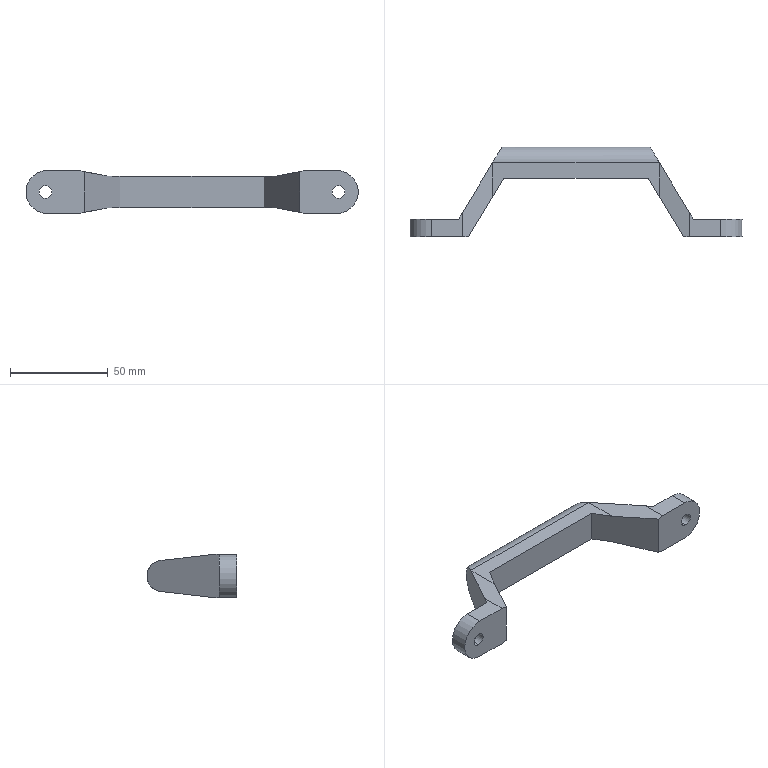Part | NX | features BREP 1 | 1 solid | 34 faces | box 170 x 46 x 22 mm | volume 38783 mm3 | plane 23 | cylinder 7 | cone 4 | commonest cylinder face diameters 6.5 x4 22 x2 16 x1
STEP:
#1=CARTESIAN_POINT('',(-75.,4.5,-3.25));
#2=VERTEX_POINT('',#1);
#3=CARTESIAN_POINT('',(-75.,4.5,3.25));
#4=VERTEX_POINT('',#3);
#5=CARTESIAN_POINT('',(-75.,4.5,0.));
#6=DIRECTION('',(0.,1.,0.));
#7=DIRECTION('',(0.,0.,1.));
#8=AXIS2_PLACEMENT_3D('',#5,#6,#7);
#9=CIRCLE('',#8,3.25);
#10=EDGE_CURVE('',#2,#4,#9,.T.);
#11=ORIENTED_EDGE('',*,*,#10,.F.);
#12=CARTESIAN_POINT('',(-75.,9.,-6.25));
#13=VERTEX_POINT('',#12);
#14=CARTESIAN_POINT('',(-75.,9.,-6.25));
#15=DIRECTION('',(0.,0.8321,-0.5547));
#16=VECTOR('',#15,1000.);
#17=LINE('',#14,#16);
#18=EDGE_CURVE('',#13,#2,#17,.F.);
#19=ORIENTED_EDGE('',*,*,#18,.F.);
#20=CARTESIAN_POINT('',(-75.,9.,6.25));
#21=VERTEX_POINT('',#20);
#22=CARTESIAN_POINT('',(-75.,9.,0.));
#23=DIRECTION('',(0.,-1.,0.));
#24=DIRECTION('',(0.,0.,1.));
#25=AXIS2_PLACEMENT_3D('',#22,#23,#24);
#26=CIRCLE('',#25,6.25);
#27=EDGE_CURVE('',#21,#13,#26,.T.);
#28=ORIENTED_EDGE('',*,*,#27,.F.);
#29=CARTESIAN_POINT('',(-75.,9.,6.25));
#30=DIRECTION('',(0.,0.8321,0.5547));
#31=VECTOR('',#30,1000.);
#32=LINE('',#29,#31);
#33=EDGE_CURVE('',#21,#4,#32,.F.);
#34=ORIENTED_EDGE('',*,*,#33,.T.);
#35=EDGE_LOOP('',(#11,#19,#28,#34));
#36=FACE_BOUND('',#35,.T.);
#37=CARTESIAN_POINT('',(-75.,9.,0.));
#38=DIRECTION('',(0.,1.,0.));
#39=DIRECTION('',(0.,0.,1.));
#40=AXIS2_PLACEMENT_3D('',#37,#38,#39);
#41=CONICAL_SURFACE('',#40,6.25,0.588);
#42=ADVANCED_FACE('',(#36),#41,.F.);
#43=CARTESIAN_POINT('',(75.,4.5,-3.25));
#44=VERTEX_POINT('',#43);
#45=CARTESIAN_POINT('',(75.,4.5,3.25));
#46=VERTEX_POINT('',#45);
#47=CARTESIAN_POINT('',(75.,4.5,0.));
#48=DIRECTION('',(0.,1.,0.));
#49=DIRECTION('',(0.,0.,1.));
#50=AXIS2_PLACEMENT_3D('',#47,#48,#49);
#51=CIRCLE('',#50,3.25);
#52=EDGE_CURVE('',#44,#46,#51,.T.);
#53=ORIENTED_EDGE('',*,*,#52,.F.);
#54=CARTESIAN_POINT('',(75.,9.,-6.25));
#55=VERTEX_POINT('',#54);
#56=CARTESIAN_POINT('',(75.,9.,-6.25));
#57=DIRECTION('',(0.,0.8321,-0.5547));
#58=VECTOR('',#57,1000.);
#59=LINE('',#56,#58);
#60=EDGE_CURVE('',#55,#44,#59,.F.);
#61=ORIENTED_EDGE('',*,*,#60,.F.);
#62=CARTESIAN_POINT('',(75.,9.,6.25));
#63=VERTEX_POINT('',#62);
#64=CARTESIAN_POINT('',(75.,9.,0.));
#65=DIRECTION('',(0.,-1.,0.));
#66=DIRECTION('',(0.,0.,1.));
#67=AXIS2_PLACEMENT_3D('',#64,#65,#66);
#68=CIRCLE('',#67,6.25);
#69=EDGE_CURVE('',#63,#55,#68,.T.);
#70=ORIENTED_EDGE('',*,*,#69,.F.);
#71=CARTESIAN_POINT('',(75.,9.,6.25));
#72=DIRECTION('',(0.,0.8321,0.5547));
#73=VECTOR('',#72,1000.);
#74=LINE('',#71,#73);
#75=EDGE_CURVE('',#63,#46,#74,.F.);
#76=ORIENTED_EDGE('',*,*,#75,.T.);
#77=EDGE_LOOP('',(#53,#61,#70,#76));
#78=FACE_BOUND('',#77,.T.);
#79=CARTESIAN_POINT('',(75.,9.,0.));
#80=DIRECTION('',(0.,1.,0.));
#81=DIRECTION('',(0.,0.,1.));
#82=AXIS2_PLACEMENT_3D('',#79,#80,#81);
#83=CONICAL_SURFACE('',#82,6.25,0.588);
#84=ADVANCED_FACE('',(#78),#83,.F.);
#85=ORIENTED_EDGE('',*,*,#10,.T.);
#86=CARTESIAN_POINT('',(-75.,0.,3.25));
#87=VERTEX_POINT('',#86);
#88=CARTESIAN_POINT('',(-75.,2.25,3.25));
#89=DIRECTION('',(0.,-1.,0.));
#90=VECTOR('',#89,1000.);
#91=LINE('',#88,#90);
#92=EDGE_CURVE('',#4,#87,#91,.T.);
#93=ORIENTED_EDGE('',*,*,#92,.T.);
#94=CARTESIAN_POINT('',(-75.,0.,-3.25));
#95=VERTEX_POINT('',#94);
#96=CARTESIAN_POINT('',(-75.,0.,0.));
#97=DIRECTION('',(0.,1.,0.));
#98=DIRECTION('',(0.,0.,-1.));
#99=AXIS2_PLACEMENT_3D('',#96,#97,#98);
#100=CIRCLE('',#99,3.25);
#101=EDGE_CURVE('',#95,#87,#100,.T.);
#102=ORIENTED_EDGE('',*,*,#101,.F.);
#103=CARTESIAN_POINT('',(-75.,2.25,-3.25));
#104=DIRECTION('',(0.,-1.,0.));
#105=VECTOR('',#104,1000.);
#106=LINE('',#103,#105);
#107=EDGE_CURVE('',#2,#95,#106,.T.);
#108=ORIENTED_EDGE('',*,*,#107,.F.);
#109=EDGE_LOOP('',(#85,#93,#102,#108));
#110=FACE_BOUND('',#109,.T.);
#111=CARTESIAN_POINT('',(-75.,2.25,0.));
#112=DIRECTION('',(0.,-1.,0.));
#113=DIRECTION('',(0.,0.,-1.));
#114=AXIS2_PLACEMENT_3D('',#111,#112,#113);
#115=CYLINDRICAL_SURFACE('',#114,3.25);
#116=ADVANCED_FACE('',(#110),#115,.F.);
#117=ORIENTED_EDGE('',*,*,#52,.T.);
#118=CARTESIAN_POINT('',(75.,0.,3.25));
#119=VERTEX_POINT('',#118);
#120=CARTESIAN_POINT('',(75.,2.25,3.25));
#121=DIRECTION('',(0.,-1.,0.));
#122=VECTOR('',#121,1000.);
#123=LINE('',#120,#122);
#124=EDGE_CURVE('',#46,#119,#123,.T.);
#125=ORIENTED_EDGE('',*,*,#124,.T.);
#126=CARTESIAN_POINT('',(75.,0.,-3.25));
#127=VERTEX_POINT('',#126);
#128=CARTESIAN_POINT('',(75.,0.,0.));
#129=DIRECTION('',(0.,1.,0.));
#130=DIRECTION('',(0.,0.,-1.));
#131=AXIS2_PLACEMENT_3D('',#128,#129,#130);
#132=CIRCLE('',#131,3.25);
#133=EDGE_CURVE('',#127,#119,#132,.T.);
#134=ORIENTED_EDGE('',*,*,#133,.F.);
#135=CARTESIAN_POINT('',(75.,2.25,-3.25));
#136=DIRECTION('',(0.,-1.,0.));
#137=VECTOR('',#136,1000.);
#138=LINE('',#135,#137);
#139=EDGE_CURVE('',#44,#127,#138,.T.);
#140=ORIENTED_EDGE('',*,*,#139,.F.);
#141=EDGE_LOOP('',(#117,#125,#134,#140));
#142=FACE_BOUND('',#141,.T.);
#143=CARTESIAN_POINT('',(75.,2.25,0.));
#144=DIRECTION('',(0.,-1.,0.));
#145=DIRECTION('',(0.,0.,-1.));
#146=AXIS2_PLACEMENT_3D('',#143,#144,#145);
#147=CYLINDRICAL_SURFACE('',#146,3.25);
#148=ADVANCED_FACE('',(#142),#147,.F.);
#149=CARTESIAN_POINT('',(-42.667,38.,-8.));
#150=VERTEX_POINT('',#149);
#151=CARTESIAN_POINT('',(-42.667,38.,8.));
#152=VERTEX_POINT('',#151);
#153=CARTESIAN_POINT('',(-42.667,38.,-8.));
#154=CARTESIAN_POINT('',(-33.053,54.,-8.));
#155=CARTESIAN_POINT('',(-33.053,54.,8.));
#156=CARTESIAN_POINT('',(-42.667,38.,8.));
#157=(BOUNDED_CURVE()B_SPLINE_CURVE(3,(#153,#154,#155,#156),.UNSPECIFIED.,.F.,.F.)B_SPLINE_CURVE_WITH_KNOTS((4,4),(4.712,7.854),.UNSPECIFIED.)CURVE()GEOMETRIC_REPRESENTATION_ITEM()RATIONAL_B_SPLINE_CURVE((1.,0.3333,0.3333,1.))REPRESENTATION_ITEM(''));
#158=EDGE_CURVE('',#150,#152,#157,.T.);
#159=ORIENTED_EDGE('',*,*,#158,.T.);
#160=CARTESIAN_POINT('',(-42.566,38.,8.));
#161=VERTEX_POINT('',#160);
#162=CARTESIAN_POINT('',(85.,38.,8.));
#163=DIRECTION('',(1.,0.,0.));
#164=VECTOR('',#163,1000.);
#165=LINE('',#162,#164);
#166=EDGE_CURVE('',#152,#161,#165,.T.);
#167=ORIENTED_EDGE('',*,*,#166,.T.);
#168=CARTESIAN_POINT('',(42.566,38.,8.));
#169=VERTEX_POINT('',#168);
#170=CARTESIAN_POINT('',(85.,38.,8.));
#171=DIRECTION('',(1.,0.,0.));
#172=VECTOR('',#171,1000.);
#173=LINE('',#170,#172);
#174=EDGE_CURVE('',#161,#169,#173,.T.);
#175=ORIENTED_EDGE('',*,*,#174,.T.);
#176=CARTESIAN_POINT('',(42.667,38.,8.));
#177=VERTEX_POINT('',#176);
#178=CARTESIAN_POINT('',(85.,38.,8.));
#179=DIRECTION('',(1.,0.,0.));
#180=VECTOR('',#179,1000.);
#181=LINE('',#178,#180);
#182=EDGE_CURVE('',#169,#177,#181,.T.);
#183=ORIENTED_EDGE('',*,*,#182,.T.);
#184=CARTESIAN_POINT('',(42.667,38.,-8.));
#185=VERTEX_POINT('',#184);
#186=CARTESIAN_POINT('',(42.667,38.,8.));
#187=CARTESIAN_POINT('',(33.053,54.,8.));
#188=CARTESIAN_POINT('',(33.053,54.,-8.));
#189=CARTESIAN_POINT('',(42.667,38.,-8.));
#190=(BOUNDED_CURVE()B_SPLINE_CURVE(3,(#186,#187,#188,#189),.UNSPECIFIED.,.F.,.F.)B_SPLINE_CURVE_WITH_KNOTS((4,4),(1.571,4.712),.UNSPECIFIED.)CURVE()GEOMETRIC_REPRESENTATION_ITEM()RATIONAL_B_SPLINE_CURVE((1.,0.3333,0.3333,1.))REPRESENTATION_ITEM(''));
#191=EDGE_CURVE('',#177,#185,#190,.T.);
#192=ORIENTED_EDGE('',*,*,#191,.T.);
#193=CARTESIAN_POINT('',(42.566,38.,-8.));
#194=VERTEX_POINT('',#193);
#195=CARTESIAN_POINT('',(85.,38.,-8.));
#196=DIRECTION('',(-1.,0.,0.));
#197=VECTOR('',#196,1000.);
#198=LINE('',#195,#197);
#199=EDGE_CURVE('',#185,#194,#198,.T.);
#200=ORIENTED_EDGE('',*,*,#199,.T.);
#201=CARTESIAN_POINT('',(-42.566,38.,-8.));
#202=VERTEX_POINT('',#201);
#203=CARTESIAN_POINT('',(85.,38.,-8.));
#204=DIRECTION('',(-1.,0.,0.));
#205=VECTOR('',#204,1000.);
#206=LINE('',#203,#205);
#207=EDGE_CURVE('',#194,#202,#206,.T.);
#208=ORIENTED_EDGE('',*,*,#207,.T.);
#209=CARTESIAN_POINT('',(85.,38.,-8.));
#210=DIRECTION('',(-1.,0.,0.));
#211=VECTOR('',#210,1000.);
#212=LINE('',#209,#211);
#213=EDGE_CURVE('',#202,#150,#212,.T.);
#214=ORIENTED_EDGE('',*,*,#213,.T.);
#215=EDGE_LOOP('',(#159,#167,#175,#183,#192,#200,#208,#214));
#216=FACE_BOUND('',#215,.T.);
#217=CARTESIAN_POINT('',(85.,38.,0.));
#218=DIRECTION('',(1.,0.,0.));
#219=DIRECTION('',(0.,0.,-1.));
#220=AXIS2_PLACEMENT_3D('',#217,#218,#219);
#221=CYLINDRICAL_SURFACE('',#220,8.);
#222=ADVANCED_FACE('',(#216),#221,.T.);
#223=CARTESIAN_POINT('',(-42.667,38.,8.02));
#224=VERTEX_POINT('',#223);
#225=CARTESIAN_POINT('',(-42.667,38.,9.9));
#226=DIRECTION('',(0.,0.,-1.));
#227=VECTOR('',#226,1000.);
#228=LINE('',#225,#227);
#229=EDGE_CURVE('',#224,#152,#228,.T.);
#230=ORIENTED_EDGE('',*,*,#229,.F.);
#231=CARTESIAN_POINT('',(-42.566,38.,8.));
#232=DIRECTION('',(0.9816,0.,-0.1908));
#233=VECTOR('',#232,1000.);
#234=LINE('',#231,#233);
#235=EDGE_CURVE('',#224,#161,#234,.T.);
#236=ORIENTED_EDGE('',*,*,#235,.T.);
#237=ORIENTED_EDGE('',*,*,#166,.F.);
#238=EDGE_LOOP('',(#230,#236,#237));
#239=FACE_BOUND('',#238,.T.);
#240=CARTESIAN_POINT('',(85.,38.,9.9));
#241=DIRECTION('',(0.,-1.,0.));
#242=DIRECTION('',(-1.,0.,0.));
#243=AXIS2_PLACEMENT_3D('',#240,#241,#242);
#244=PLANE('',#243);
#245=ADVANCED_FACE('',(#239),#244,.F.);
#246=CARTESIAN_POINT('',(-58.,12.482,-11.));
#247=VERTEX_POINT('',#246);
#248=CARTESIAN_POINT('',(-60.092,9.,-11.));
#249=VERTEX_POINT('',#248);
#250=CARTESIAN_POINT('',(-37.86,46.,-11.));
#251=DIRECTION('',(-0.515,-0.8572,0.));
#252=VECTOR('',#251,1000.);
#253=LINE('',#250,#252);
#254=EDGE_CURVE('',#247,#249,#253,.T.);
#255=ORIENTED_EDGE('',*,*,#254,.T.);
#256=CARTESIAN_POINT('',(-60.092,9.,11.));
#257=VERTEX_POINT('',#256);
#258=CARTESIAN_POINT('',(-60.092,9.,11.));
#259=DIRECTION('',(0.,0.,1.));
#260=VECTOR('',#259,1000.);
#261=LINE('',#258,#260);
#262=EDGE_CURVE('',#249,#257,#261,.T.);
#263=ORIENTED_EDGE('',*,*,#262,.T.);
#264=CARTESIAN_POINT('',(-58.,12.482,11.));
#265=VERTEX_POINT('',#264);
#266=CARTESIAN_POINT('',(-37.86,46.,11.));
#267=DIRECTION('',(0.515,0.8572,0.));
#268=VECTOR('',#267,1000.);
#269=LINE('',#266,#268);
#270=EDGE_CURVE('',#257,#265,#269,.T.);
#271=ORIENTED_EDGE('',*,*,#270,.T.);
#272=CARTESIAN_POINT('',(-58.,12.482,11.));
#273=DIRECTION('',(0.5125,0.8529,-0.09962));
#274=VECTOR('',#273,1000.);
#275=LINE('',#272,#274);
#276=EDGE_CURVE('',#265,#224,#275,.T.);
#277=ORIENTED_EDGE('',*,*,#276,.T.);
#278=ORIENTED_EDGE('',*,*,#229,.T.);
#279=ORIENTED_EDGE('',*,*,#158,.F.);
#280=CARTESIAN_POINT('',(-42.667,38.,-8.02));
#281=VERTEX_POINT('',#280);
#282=CARTESIAN_POINT('',(-42.667,38.,11.));
#283=DIRECTION('',(0.,0.,-1.));
#284=VECTOR('',#283,1000.);
#285=LINE('',#282,#284);
#286=EDGE_CURVE('',#150,#281,#285,.T.);
#287=ORIENTED_EDGE('',*,*,#286,.T.);
#288=CARTESIAN_POINT('',(-42.667,38.,-8.02));
#289=DIRECTION('',(-0.5125,-0.8529,-0.09962));
#290=VECTOR('',#289,1000.);
#291=LINE('',#288,#290);
#292=EDGE_CURVE('',#281,#247,#291,.T.);
#293=ORIENTED_EDGE('',*,*,#292,.T.);
#294=EDGE_LOOP('',(#255,#263,#271,#277,#278,#279,#287,#293));
#295=FACE_BOUND('',#294,.T.);
#296=CARTESIAN_POINT('',(-37.86,46.,11.));
#297=DIRECTION('',(-0.8572,0.515,0.));
#298=DIRECTION('',(0.,0.,1.));
#299=AXIS2_PLACEMENT_3D('',#296,#297,#298);
#300=PLANE('',#299);
#301=ADVANCED_FACE('',(#295),#300,.T.);
#302=CARTESIAN_POINT('',(-42.667,38.,-8.02));
#303=DIRECTION('',(0.9816,0.,0.1908));
#304=VECTOR('',#303,1000.);
#305=LINE('',#302,#304);
#306=EDGE_CURVE('',#281,#202,#305,.T.);
#307=ORIENTED_EDGE('',*,*,#306,.F.);
#308=ORIENTED_EDGE('',*,*,#286,.F.);
#309=ORIENTED_EDGE('',*,*,#213,.F.);
#310=EDGE_LOOP('',(#307,#308,#309));
#311=FACE_BOUND('',#310,.T.);
#312=CARTESIAN_POINT('',(85.,38.,-8.));
#313=DIRECTION('',(0.,-1.,0.));
#314=DIRECTION('',(0.,0.,-1.));
#315=AXIS2_PLACEMENT_3D('',#312,#313,#314);
#316=PLANE('',#315);
#317=ADVANCED_FACE('',(#311),#316,.F.);
#318=CARTESIAN_POINT('',(36.974,30.,-8.));
#319=VERTEX_POINT('',#318);
#320=CARTESIAN_POINT('',(42.566,20.693,-8.));
#321=VERTEX_POINT('',#320);
#322=CARTESIAN_POINT('',(36.974,30.,-8.));
#323=DIRECTION('',(0.515,-0.8572,0.));
#324=VECTOR('',#323,1000.);
#325=LINE('',#322,#324);
#326=EDGE_CURVE('',#319,#321,#325,.T.);
#327=ORIENTED_EDGE('',*,*,#326,.F.);
#328=CARTESIAN_POINT('',(-36.974,30.,-8.));
#329=VERTEX_POINT('',#328);
#330=CARTESIAN_POINT('',(-42.566,30.,-8.));
#331=DIRECTION('',(1.,0.,0.));
#332=VECTOR('',#331,1000.);
#333=LINE('',#330,#332);
#334=EDGE_CURVE('',#329,#319,#333,.T.);
#335=ORIENTED_EDGE('',*,*,#334,.F.);
#336=CARTESIAN_POINT('',(-42.566,20.693,-8.));
#337=VERTEX_POINT('',#336);
#338=CARTESIAN_POINT('',(-42.566,20.693,-8.));
#339=DIRECTION('',(0.515,0.8572,0.));
#340=VECTOR('',#339,1000.);
#341=LINE('',#338,#340);
#342=EDGE_CURVE('',#337,#329,#341,.T.);
#343=ORIENTED_EDGE('',*,*,#342,.F.);
#344=CARTESIAN_POINT('',(-42.566,46.,-8.));
#345=DIRECTION('',(0.,-1.,0.));
#346=VECTOR('',#345,1000.);
#347=LINE('',#344,#346);
#348=EDGE_CURVE('',#202,#337,#347,.T.);
#349=ORIENTED_EDGE('',*,*,#348,.F.);
#350=ORIENTED_EDGE('',*,*,#207,.F.);
#351=CARTESIAN_POINT('',(42.566,46.,-8.));
#352=DIRECTION('',(0.,1.,0.));
#353=VECTOR('',#352,1000.);
#354=LINE('',#351,#353);
#355=EDGE_CURVE('',#321,#194,#354,.T.);
#356=ORIENTED_EDGE('',*,*,#355,.F.);
#357=EDGE_LOOP('',(#327,#335,#343,#349,#350,#356));
#358=FACE_BOUND('',#357,.T.);
#359=CARTESIAN_POINT('',(-42.566,46.,-8.));
#360=DIRECTION('',(0.,0.,1.));
#361=DIRECTION('',(1.,0.,0.));
#362=AXIS2_PLACEMENT_3D('',#359,#360,#361);
#363=PLANE('',#362);
#364=ADVANCED_FACE('',(#358),#363,.F.);
#365=ORIENTED_EDGE('',*,*,#199,.F.);
#366=CARTESIAN_POINT('',(42.667,38.,-8.02));
#367=VERTEX_POINT('',#366);
#368=CARTESIAN_POINT('',(42.667,38.,-8.));
#369=DIRECTION('',(0.,0.,1.));
#370=VECTOR('',#369,1000.);
#371=LINE('',#368,#370);
#372=EDGE_CURVE('',#367,#185,#371,.T.);
#373=ORIENTED_EDGE('',*,*,#372,.F.);
#374=CARTESIAN_POINT('',(42.566,38.,-8.));
#375=DIRECTION('',(0.9816,0.,-0.1908));
#376=VECTOR('',#375,1000.);
#377=LINE('',#374,#376);
#378=EDGE_CURVE('',#194,#367,#377,.T.);
#379=ORIENTED_EDGE('',*,*,#378,.F.);
#380=EDGE_LOOP('',(#365,#373,#379));
#381=FACE_BOUND('',#380,.T.);
#382=CARTESIAN_POINT('',(85.,38.,-8.));
#383=DIRECTION('',(0.,-1.,0.));
#384=DIRECTION('',(0.,0.,-1.));
#385=AXIS2_PLACEMENT_3D('',#382,#383,#384);
#386=PLANE('',#385);
#387=ADVANCED_FACE('',(#381),#386,.F.);
#388=CARTESIAN_POINT('',(60.092,9.,-11.));
#389=VERTEX_POINT('',#388);
#390=CARTESIAN_POINT('',(58.,12.482,-11.));
#391=VERTEX_POINT('',#390);
#392=CARTESIAN_POINT('',(60.092,9.,-11.));
#393=DIRECTION('',(-0.515,0.8572,0.));
#394=VECTOR('',#393,1000.);
#395=LINE('',#392,#394);
#396=EDGE_CURVE('',#389,#391,#395,.T.);
#397=ORIENTED_EDGE('',*,*,#396,.T.);
#398=CARTESIAN_POINT('',(58.,12.482,-11.));
#399=DIRECTION('',(-0.5125,0.8529,0.09962));
#400=VECTOR('',#399,1000.);
#401=LINE('',#398,#400);
#402=EDGE_CURVE('',#391,#367,#401,.T.);
#403=ORIENTED_EDGE('',*,*,#402,.T.);
#404=ORIENTED_EDGE('',*,*,#372,.T.);
#405=ORIENTED_EDGE('',*,*,#191,.F.);
#406=CARTESIAN_POINT('',(42.667,38.,8.02));
#407=VERTEX_POINT('',#406);
#408=CARTESIAN_POINT('',(42.667,38.,11.));
#409=DIRECTION('',(0.,0.,1.));
#410=VECTOR('',#409,1000.);
#411=LINE('',#408,#410);
#412=EDGE_CURVE('',#177,#407,#411,.T.);
#413=ORIENTED_EDGE('',*,*,#412,.T.);
#414=CARTESIAN_POINT('',(58.,12.482,11.));
#415=VERTEX_POINT('',#414);
#416=CARTESIAN_POINT('',(42.667,38.,8.02));
#417=DIRECTION('',(0.5125,-0.8529,0.09962));
#418=VECTOR('',#417,1000.);
#419=LINE('',#416,#418);
#420=EDGE_CURVE('',#407,#415,#419,.T.);
#421=ORIENTED_EDGE('',*,*,#420,.T.);
#422=CARTESIAN_POINT('',(60.092,9.,11.));
#423=VERTEX_POINT('',#422);
#424=CARTESIAN_POINT('',(60.092,9.,11.));
#425=DIRECTION('',(0.515,-0.8572,0.));
#426=VECTOR('',#425,1000.);
#427=LINE('',#424,#426);
#428=EDGE_CURVE('',#415,#423,#427,.T.);
#429=ORIENTED_EDGE('',*,*,#428,.T.);
#430=CARTESIAN_POINT('',(60.092,9.,11.));
#431=DIRECTION('',(0.,0.,-1.));
#432=VECTOR('',#431,1000.);
#433=LINE('',#430,#432);
#434=EDGE_CURVE('',#423,#389,#433,.T.);
#435=ORIENTED_EDGE('',*,*,#434,.T.);
#436=EDGE_LOOP('',(#397,#403,#404,#405,#413,#421,#429,#435));
#437=FACE_BOUND('',#436,.T.);
#438=CARTESIAN_POINT('',(60.092,9.,11.));
#439=DIRECTION('',(0.8572,0.515,0.));
#440=DIRECTION('',(0.,0.,-1.));
#441=AXIS2_PLACEMENT_3D('',#438,#439,#440);
#442=PLANE('',#441);
#443=ADVANCED_FACE('',(#437),#442,.T.);
#444=ORIENTED_EDGE('',*,*,#182,.F.);
#445=CARTESIAN_POINT('',(42.667,38.,8.02));
#446=DIRECTION('',(-0.9816,0.,-0.1908));
#447=VECTOR('',#446,1000.);
#448=LINE('',#445,#447);
#449=EDGE_CURVE('',#407,#169,#448,.T.);
#450=ORIENTED_EDGE('',*,*,#449,.F.);
#451=ORIENTED_EDGE('',*,*,#412,.F.);
#452=EDGE_LOOP('',(#444,#450,#451));
#453=FACE_BOUND('',#452,.T.);
#454=CARTESIAN_POINT('',(85.,38.,9.9));
#455=DIRECTION('',(0.,-1.,0.));
#456=DIRECTION('',(-1.,0.,0.));
#457=AXIS2_PLACEMENT_3D('',#454,#455,#456);
#458=PLANE('',#457);
#459=ADVANCED_FACE('',(#453),#458,.F.);
#460=CARTESIAN_POINT('',(-36.974,30.,8.));
#461=VERTEX_POINT('',#460);
#462=CARTESIAN_POINT('',(-42.566,20.693,8.));
#463=VERTEX_POINT('',#462);
#464=CARTESIAN_POINT('',(-36.974,30.,8.));
#465=DIRECTION('',(-0.515,-0.8572,0.));
#466=VECTOR('',#465,1000.);
#467=LINE('',#464,#466);
#468=EDGE_CURVE('',#461,#463,#467,.T.);
#469=ORIENTED_EDGE('',*,*,#468,.F.);
#470=CARTESIAN_POINT('',(36.974,30.,8.));
#471=VERTEX_POINT('',#470);
#472=CARTESIAN_POINT('',(42.566,30.,8.));
#473=DIRECTION('',(-1.,0.,0.));
#474=VECTOR('',#473,1000.);
#475=LINE('',#472,#474);
#476=EDGE_CURVE('',#471,#461,#475,.T.);
#477=ORIENTED_EDGE('',*,*,#476,.F.);
#478=CARTESIAN_POINT('',(42.566,20.693,8.));
#479=VERTEX_POINT('',#478);
#480=CARTESIAN_POINT('',(42.566,20.693,8.));
#481=DIRECTION('',(-0.515,0.8572,0.));
#482=VECTOR('',#481,1000.);
#483=LINE('',#480,#482);
#484=EDGE_CURVE('',#479,#471,#483,.T.);
#485=ORIENTED_EDGE('',*,*,#484,.F.);
#486=CARTESIAN_POINT('',(42.566,46.,8.));
#487=DIRECTION('',(0.,-1.,0.));
#488=VECTOR('',#487,1000.);
#489=LINE('',#486,#488);
#490=EDGE_CURVE('',#169,#479,#489,.T.);
#491=ORIENTED_EDGE('',*,*,#490,.F.);
#492=ORIENTED_EDGE('',*,*,#174,.F.);
#493=CARTESIAN_POINT('',(-42.566,46.,8.));
#494=DIRECTION('',(0.,1.,0.));
#495=VECTOR('',#494,1000.);
#496=LINE('',#493,#495);
#497=EDGE_CURVE('',#463,#161,#496,.T.);
#498=ORIENTED_EDGE('',*,*,#497,.F.);
#499=EDGE_LOOP('',(#469,#477,#485,#491,#492,#498));
#500=FACE_BOUND('',#499,.T.);
#501=CARTESIAN_POINT('',(42.566,46.,8.));
#502=DIRECTION('',(0.,0.,-1.));
#503=DIRECTION('',(0.,-1.,0.));
#504=AXIS2_PLACEMENT_3D('',#501,#502,#503);
#505=PLANE('',#504);
#506=ADVANCED_FACE('',(#500),#505,.F.);
#507=CARTESIAN_POINT('',(-74.,9.,-11.));
#508=VERTEX_POINT('',#507);
#509=CARTESIAN_POINT('',(-74.,9.,11.));
#510=VERTEX_POINT('',#509);
#511=CARTESIAN_POINT('',(-74.,9.,0.));
#512=DIRECTION('',(0.,1.,0.));
#513=DIRECTION('',(0.,0.,-1.));
#514=AXIS2_PLACEMENT_3D('',#511,#512,#513);
#515=CIRCLE('',#514,11.);
#516=EDGE_CURVE('',#508,#510,#515,.T.);
#517=ORIENTED_EDGE('',*,*,#516,.T.);
#518=CARTESIAN_POINT('',(-60.092,9.,11.));
#519=DIRECTION('',(1.,0.,0.));
#520=VECTOR('',#519,1000.);
#521=LINE('',#518,#520);
#522=EDGE_CURVE('',#510,#257,#521,.T.);
#523=ORIENTED_EDGE('',*,*,#522,.T.);
#524=ORIENTED_EDGE('',*,*,#262,.F.);
#525=CARTESIAN_POINT('',(-60.092,9.,-11.));
#526=DIRECTION('',(-1.,0.,0.));
#527=VECTOR('',#526,1000.);
#528=LINE('',#525,#527);
#529=EDGE_CURVE('',#249,#508,#528,.T.);
#530=ORIENTED_EDGE('',*,*,#529,.T.);
#531=EDGE_LOOP('',(#517,#523,#524,#530));
#532=FACE_BOUND('',#531,.T.);
#533=ORIENTED_EDGE('',*,*,#27,.T.);
#534=CARTESIAN_POINT('',(-75.,9.,0.));
#535=DIRECTION('',(0.,-1.,0.));
#536=DIRECTION('',(0.,0.,1.));
#537=AXIS2_PLACEMENT_3D('',#534,#535,#536);
#538=CIRCLE('',#537,6.25);
#539=EDGE_CURVE('',#13,#21,#538,.T.);
#540=ORIENTED_EDGE('',*,*,#539,.T.);
#541=EDGE_LOOP('',(#533,#540));
#542=FACE_BOUND('',#541,.T.);
#543=CARTESIAN_POINT('',(-60.092,9.,11.));
#544=DIRECTION('',(0.,1.,0.));
#545=DIRECTION('',(1.,0.,0.));
#546=AXIS2_PLACEMENT_3D('',#543,#544,#545);
#547=PLANE('',#546);
#548=ADVANCED_FACE('',(#532,#542),#547,.T.);
#549=ORIENTED_EDGE('',*,*,#254,.F.);
#550=CARTESIAN_POINT('',(-58.,0.,-11.));
#551=VERTEX_POINT('',#550);
#552=CARTESIAN_POINT('',(-58.,0.,-11.));
#553=DIRECTION('',(0.,1.,0.));
#554=VECTOR('',#553,1000.);
#555=LINE('',#552,#554);
#556=EDGE_CURVE('',#551,#247,#555,.T.);
#557=ORIENTED_EDGE('',*,*,#556,.F.);
#558=CARTESIAN_POINT('',(-74.,0.,-11.));
#559=VERTEX_POINT('',#558);
#560=CARTESIAN_POINT('',(0.,0.,-11.));
#561=DIRECTION('',(1.,0.,0.));
#562=VECTOR('',#561,1000.);
#563=LINE('',#560,#562);
#564=EDGE_CURVE('',#559,#551,#563,.T.);
#565=ORIENTED_EDGE('',*,*,#564,.F.);
#566=CARTESIAN_POINT('',(-74.,0.,-11.));
#567=DIRECTION('',(0.,-1.,0.));
#568=VECTOR('',#567,1000.);
#569=LINE('',#566,#568);
#570=EDGE_CURVE('',#508,#559,#569,.T.);
#571=ORIENTED_EDGE('',*,*,#570,.F.);
#572=ORIENTED_EDGE('',*,*,#529,.F.);
#573=EDGE_LOOP('',(#549,#557,#565,#571,#572));
#574=FACE_BOUND('',#573,.T.);
#575=CARTESIAN_POINT('',(0.,0.,-11.));
#576=DIRECTION('',(0.,0.,1.));
#577=DIRECTION('',(1.,0.,0.));
#578=AXIS2_PLACEMENT_3D('',#575,#576,#577);
#579=PLANE('',#578);
#580=ADVANCED_FACE('',(#574),#579,.F.);
#581=CARTESIAN_POINT('',(-55.,0.,-10.417));
#582=VERTEX_POINT('',#581);
#583=CARTESIAN_POINT('',(-55.,0.,-10.417));
#584=DIRECTION('',(0.5125,0.8529,0.09962));
#585=VECTOR('',#584,1000.);
#586=LINE('',#583,#585);
#587=EDGE_CURVE('',#582,#337,#586,.T.);
#588=ORIENTED_EDGE('',*,*,#587,.F.);
#589=CARTESIAN_POINT('',(-58.,0.,-11.));
#590=DIRECTION('',(0.9816,0.,0.1908));
#591=VECTOR('',#590,1000.);
#592=LINE('',#589,#591);
#593=EDGE_CURVE('',#551,#582,#592,.T.);
#594=ORIENTED_EDGE('',*,*,#593,.F.);
#595=ORIENTED_EDGE('',*,*,#556,.T.);
#596=ORIENTED_EDGE('',*,*,#292,.F.);
#597=ORIENTED_EDGE('',*,*,#306,.T.);
#598=ORIENTED_EDGE('',*,*,#348,.T.);
#599=EDGE_LOOP('',(#588,#594,#595,#596,#597,#598));
#600=FACE_BOUND('',#599,.T.);
#601=CARTESIAN_POINT('',(-58.,46.,-11.));
#602=DIRECTION('',(-0.1908,0.,0.9816));
#603=DIRECTION('',(0.,1.,0.));
#604=AXIS2_PLACEMENT_3D('',#601,#602,#603);
#605=PLANE('',#604);
#606=ADVANCED_FACE('',(#600),#605,.F.);
#607=CARTESIAN_POINT('',(-58.,0.,11.));
#608=VERTEX_POINT('',#607);
#609=CARTESIAN_POINT('',(-58.,46.,11.));
#610=DIRECTION('',(0.,1.,0.));
#611=VECTOR('',#610,1000.);
#612=LINE('',#609,#611);
#613=EDGE_CURVE('',#608,#265,#612,.T.);
#614=ORIENTED_EDGE('',*,*,#613,.F.);
#615=CARTESIAN_POINT('',(-55.,0.,10.417));
#616=VERTEX_POINT('',#615);
#617=CARTESIAN_POINT('',(-42.566,0.,8.));
#618=DIRECTION('',(-0.9816,0.,0.1908));
#619=VECTOR('',#618,1000.);
#620=LINE('',#617,#619);
#621=EDGE_CURVE('',#616,#608,#620,.T.);
#622=ORIENTED_EDGE('',*,*,#621,.F.);
#623=CARTESIAN_POINT('',(-42.566,20.693,8.));
#624=DIRECTION('',(-0.5125,-0.8529,0.09962));
#625=VECTOR('',#624,1000.);
#626=LINE('',#623,#625);
#627=EDGE_CURVE('',#463,#616,#626,.T.);
#628=ORIENTED_EDGE('',*,*,#627,.F.);
#629=ORIENTED_EDGE('',*,*,#497,.T.);
#630=ORIENTED_EDGE('',*,*,#235,.F.);
#631=ORIENTED_EDGE('',*,*,#276,.F.);
#632=EDGE_LOOP('',(#614,#622,#628,#629,#630,#631));
#633=FACE_BOUND('',#632,.T.);
#634=CARTESIAN_POINT('',(-42.566,46.,8.));
#635=DIRECTION('',(-0.1908,0.,-0.9816));
#636=DIRECTION('',(-0.9816,0.,0.1908));
#637=AXIS2_PLACEMENT_3D('',#634,#635,#636);
#638=PLANE('',#637);
#639=ADVANCED_FACE('',(#633),#638,.F.);
#640=CARTESIAN_POINT('',(-74.,0.,11.));
#641=VERTEX_POINT('',#640);
#642=CARTESIAN_POINT('',(0.,0.,11.));
#643=DIRECTION('',(1.,0.,0.));
#644=VECTOR('',#643,1000.);
#645=LINE('',#642,#644);
#646=EDGE_CURVE('',#641,#608,#645,.T.);
#647=ORIENTED_EDGE('',*,*,#646,.T.);
#648=ORIENTED_EDGE('',*,*,#613,.T.);
#649=ORIENTED_EDGE('',*,*,#270,.F.);
#650=ORIENTED_EDGE('',*,*,#522,.F.);
#651=CARTESIAN_POINT('',(-74.,0.,11.));
#652=DIRECTION('',(0.,-1.,0.));
#653=VECTOR('',#652,1000.);
#654=LINE('',#651,#653);
#655=EDGE_CURVE('',#510,#641,#654,.T.);
#656=ORIENTED_EDGE('',*,*,#655,.T.);
#657=EDGE_LOOP('',(#647,#648,#649,#650,#656));
#658=FACE_BOUND('',#657,.T.);
#659=CARTESIAN_POINT('',(0.,0.,11.));
#660=DIRECTION('',(0.,0.,1.));
#661=DIRECTION('',(1.,0.,0.));
#662=AXIS2_PLACEMENT_3D('',#659,#660,#661);
#663=PLANE('',#662);
#664=ADVANCED_FACE('',(#658),#663,.T.);
#665=CARTESIAN_POINT('',(58.,0.,-11.));
#666=VERTEX_POINT('',#665);
#667=CARTESIAN_POINT('',(58.,46.,-11.));
#668=DIRECTION('',(0.,1.,0.));
#669=VECTOR('',#668,1000.);
#670=LINE('',#667,#669);
#671=EDGE_CURVE('',#666,#391,#670,.T.);
#672=ORIENTED_EDGE('',*,*,#671,.F.);
#673=CARTESIAN_POINT('',(55.,0.,-10.417));
#674=VERTEX_POINT('',#673);
#675=CARTESIAN_POINT('',(42.566,0.,-8.));
#676=DIRECTION('',(0.9816,0.,-0.1908));
#677=VECTOR('',#676,1000.);
#678=LINE('',#675,#677);
#679=EDGE_CURVE('',#674,#666,#678,.T.);
#680=ORIENTED_EDGE('',*,*,#679,.F.);
#681=CARTESIAN_POINT('',(42.566,20.693,-8.));
#682=DIRECTION('',(0.5125,-0.8529,-0.09962));
#683=VECTOR('',#682,1000.);
#684=LINE('',#681,#683);
#685=EDGE_CURVE('',#321,#674,#684,.T.);
#686=ORIENTED_EDGE('',*,*,#685,.F.);
#687=ORIENTED_EDGE('',*,*,#355,.T.);
#688=ORIENTED_EDGE('',*,*,#378,.T.);
#689=ORIENTED_EDGE('',*,*,#402,.F.);
#690=EDGE_LOOP('',(#672,#680,#686,#687,#688,#689));
#691=FACE_BOUND('',#690,.T.);
#692=CARTESIAN_POINT('',(42.566,46.,-8.));
#693=DIRECTION('',(0.1908,0.,0.9816));
#694=DIRECTION('',(0.,-1.,0.));
#695=AXIS2_PLACEMENT_3D('',#692,#693,#694);
#696=PLANE('',#695);
#697=ADVANCED_FACE('',(#691),#696,.F.);
#698=CARTESIAN_POINT('',(36.974,30.,11.));
#699=DIRECTION('',(0.,0.,-1.));
#700=VECTOR('',#699,1000.);
#701=LINE('',#698,#700);
#702=EDGE_CURVE('',#471,#319,#701,.T.);
#703=ORIENTED_EDGE('',*,*,#702,.T.);
#704=ORIENTED_EDGE('',*,*,#326,.T.);
#705=ORIENTED_EDGE('',*,*,#685,.T.);
#706=CARTESIAN_POINT('',(55.,0.,10.417));
#707=VERTEX_POINT('',#706);
#708=CARTESIAN_POINT('',(55.,0.,11.));
#709=DIRECTION('',(0.,0.,1.));
#710=VECTOR('',#709,1000.);
#711=LINE('',#708,#710);
#712=EDGE_CURVE('',#674,#707,#711,.T.);
#713=ORIENTED_EDGE('',*,*,#712,.T.);
#714=CARTESIAN_POINT('',(55.,0.,10.417));
#715=DIRECTION('',(-0.5125,0.8529,-0.09962));
#716=VECTOR('',#715,1000.);
#717=LINE('',#714,#716);
#718=EDGE_CURVE('',#707,#479,#717,.T.);
#719=ORIENTED_EDGE('',*,*,#718,.T.);
#720=ORIENTED_EDGE('',*,*,#484,.T.);
#721=EDGE_LOOP('',(#703,#704,#705,#713,#719,#720));
#722=FACE_BOUND('',#721,.T.);
#723=CARTESIAN_POINT('',(36.974,30.,11.));
#724=DIRECTION('',(-0.8572,-0.515,0.));
#725=DIRECTION('',(-0.515,0.8572,0.));
#726=AXIS2_PLACEMENT_3D('',#723,#724,#725);
#727=PLANE('',#726);
#728=ADVANCED_FACE('',(#722),#727,.T.);
#729=ORIENTED_EDGE('',*,*,#476,.T.);
#730=CARTESIAN_POINT('',(-36.974,30.,11.));
#731=DIRECTION('',(0.,0.,-1.));
#732=VECTOR('',#731,1000.);
#733=LINE('',#730,#732);
#734=EDGE_CURVE('',#461,#329,#733,.T.);
#735=ORIENTED_EDGE('',*,*,#734,.T.);
#736=ORIENTED_EDGE('',*,*,#334,.T.);
#737=ORIENTED_EDGE('',*,*,#702,.F.);
#738=EDGE_LOOP('',(#729,#735,#736,#737));
#739=FACE_BOUND('',#738,.T.);
#740=CARTESIAN_POINT('',(-36.974,30.,11.));
#741=DIRECTION('',(0.,-1.,0.));
#742=DIRECTION('',(0.,0.,-1.));
#743=AXIS2_PLACEMENT_3D('',#740,#741,#742);
#744=PLANE('',#743);
#745=ADVANCED_FACE('',(#739),#744,.T.);
#746=ORIENTED_EDGE('',*,*,#587,.T.);
#747=ORIENTED_EDGE('',*,*,#342,.T.);
#748=ORIENTED_EDGE('',*,*,#734,.F.);
#749=ORIENTED_EDGE('',*,*,#468,.T.);
#750=ORIENTED_EDGE('',*,*,#627,.T.);
#751=CARTESIAN_POINT('',(-55.,0.,11.));
#752=DIRECTION('',(0.,0.,-1.));
#753=VECTOR('',#752,1000.);
#754=LINE('',#751,#753);
#755=EDGE_CURVE('',#616,#582,#754,.T.);
#756=ORIENTED_EDGE('',*,*,#755,.T.);
#757=EDGE_LOOP('',(#746,#747,#748,#749,#750,#756));
#758=FACE_BOUND('',#757,.T.);
#759=CARTESIAN_POINT('',(-55.,0.,11.));
#760=DIRECTION('',(0.8572,-0.515,0.));
#761=DIRECTION('',(0.,0.,-1.));
#762=AXIS2_PLACEMENT_3D('',#759,#760,#761);
#763=PLANE('',#762);
#764=ADVANCED_FACE('',(#758),#763,.T.);
#765=ORIENTED_EDGE('',*,*,#671,.T.);
#766=ORIENTED_EDGE('',*,*,#396,.F.);
#767=CARTESIAN_POINT('',(74.,9.,-11.));
#768=VERTEX_POINT('',#767);
#769=CARTESIAN_POINT('',(0.,9.,-11.));
#770=DIRECTION('',(-1.,0.,0.));
#771=VECTOR('',#770,1000.);
#772=LINE('',#769,#771);
#773=EDGE_CURVE('',#768,#389,#772,.T.);
#774=ORIENTED_EDGE('',*,*,#773,.F.);
#775=CARTESIAN_POINT('',(74.,0.,-11.));
#776=VERTEX_POINT('',#775);
#777=CARTESIAN_POINT('',(74.,0.,-11.));
#778=DIRECTION('',(0.,1.,0.));
#779=VECTOR('',#778,1000.);
#780=LINE('',#777,#779);
#781=EDGE_CURVE('',#776,#768,#780,.T.);
#782=ORIENTED_EDGE('',*,*,#781,.F.);
#783=CARTESIAN_POINT('',(0.,0.,-11.));
#784=DIRECTION('',(1.,0.,0.));
#785=VECTOR('',#784,1000.);
#786=LINE('',#783,#785);
#787=EDGE_CURVE('',#666,#776,#786,.T.);
#788=ORIENTED_EDGE('',*,*,#787,.F.);
#789=EDGE_LOOP('',(#765,#766,#774,#782,#788));
#790=FACE_BOUND('',#789,.T.);
#791=CARTESIAN_POINT('',(0.,0.,-11.));
#792=DIRECTION('',(0.,0.,1.));
#793=DIRECTION('',(1.,0.,0.));
#794=AXIS2_PLACEMENT_3D('',#791,#792,#793);
#795=PLANE('',#794);
#796=ADVANCED_FACE('',(#790),#795,.F.);
#797=CARTESIAN_POINT('',(74.,9.,11.));
#798=VERTEX_POINT('',#797);
#799=CARTESIAN_POINT('',(74.,9.,0.));
#800=DIRECTION('',(0.,1.,0.));
#801=DIRECTION('',(0.,0.,-1.));
#802=AXIS2_PLACEMENT_3D('',#799,#800,#801);
#803=CIRCLE('',#802,11.);
#804=EDGE_CURVE('',#798,#768,#803,.T.);
#805=ORIENTED_EDGE('',*,*,#804,.T.);
#806=ORIENTED_EDGE('',*,*,#773,.T.);
#807=ORIENTED_EDGE('',*,*,#434,.F.);
#808=CARTESIAN_POINT('',(85.,9.,11.));
#809=DIRECTION('',(1.,0.,0.));
#810=VECTOR('',#809,1000.);
#811=LINE('',#808,#810);
#812=EDGE_CURVE('',#423,#798,#811,.T.);
#813=ORIENTED_EDGE('',*,*,#812,.T.);
#814=EDGE_LOOP('',(#805,#806,#807,#813));
#815=FACE_BOUND('',#814,.T.);
#816=ORIENTED_EDGE('',*,*,#69,.T.);
#817=CARTESIAN_POINT('',(75.,9.,0.));
#818=DIRECTION('',(0.,-1.,0.));
#819=DIRECTION('',(0.,0.,1.));
#820=AXIS2_PLACEMENT_3D('',#817,#818,#819);
#821=CIRCLE('',#820,6.25);
#822=EDGE_CURVE('',#55,#63,#821,.T.);
#823=ORIENTED_EDGE('',*,*,#822,.T.);
#824=EDGE_LOOP('',(#816,#823));
#825=FACE_BOUND('',#824,.T.);
#826=CARTESIAN_POINT('',(85.,9.,11.));
#827=DIRECTION('',(0.,1.,0.));
#828=DIRECTION('',(1.,0.,0.));
#829=AXIS2_PLACEMENT_3D('',#826,#827,#828);
#830=PLANE('',#829);
#831=ADVANCED_FACE('',(#815,#825),#830,.T.);
#832=ORIENTED_EDGE('',*,*,#812,.F.);
#833=ORIENTED_EDGE('',*,*,#428,.F.);
#834=CARTESIAN_POINT('',(58.,0.,11.));
#835=VERTEX_POINT('',#834);
#836=CARTESIAN_POINT('',(58.,0.,11.));
#837=DIRECTION('',(0.,-1.,0.));
#838=VECTOR('',#837,1000.);
#839=LINE('',#836,#838);
#840=EDGE_CURVE('',#415,#835,#839,.T.);
#841=ORIENTED_EDGE('',*,*,#840,.T.);
#842=CARTESIAN_POINT('',(74.,0.,11.));
#843=VERTEX_POINT('',#842);
#844=CARTESIAN_POINT('',(0.,0.,11.));
#845=DIRECTION('',(1.,0.,0.));
#846=VECTOR('',#845,1000.);
#847=LINE('',#844,#846);
#848=EDGE_CURVE('',#835,#843,#847,.T.);
#849=ORIENTED_EDGE('',*,*,#848,.T.);
#850=CARTESIAN_POINT('',(74.,0.,11.));
#851=DIRECTION('',(0.,1.,0.));
#852=VECTOR('',#851,1000.);
#853=LINE('',#850,#852);
#854=EDGE_CURVE('',#843,#798,#853,.T.);
#855=ORIENTED_EDGE('',*,*,#854,.T.);
#856=EDGE_LOOP('',(#832,#833,#841,#849,#855));
#857=FACE_BOUND('',#856,.T.);
#858=CARTESIAN_POINT('',(0.,0.,11.));
#859=DIRECTION('',(0.,0.,1.));
#860=DIRECTION('',(1.,0.,0.));
#861=AXIS2_PLACEMENT_3D('',#858,#859,#860);
#862=PLANE('',#861);
#863=ADVANCED_FACE('',(#857),#862,.T.);
#864=ORIENTED_EDGE('',*,*,#718,.F.);
#865=CARTESIAN_POINT('',(58.,0.,11.));
#866=DIRECTION('',(-0.9816,0.,-0.1908));
#867=VECTOR('',#866,1000.);
#868=LINE('',#865,#867);
#869=EDGE_CURVE('',#835,#707,#868,.T.);
#870=ORIENTED_EDGE('',*,*,#869,.F.);
#871=ORIENTED_EDGE('',*,*,#840,.F.);
#872=ORIENTED_EDGE('',*,*,#420,.F.);
#873=ORIENTED_EDGE('',*,*,#449,.T.);
#874=ORIENTED_EDGE('',*,*,#490,.T.);
#875=EDGE_LOOP('',(#864,#870,#871,#872,#873,#874));
#876=FACE_BOUND('',#875,.T.);
#877=CARTESIAN_POINT('',(58.,46.,11.));
#878=DIRECTION('',(0.1908,0.,-0.9816));
#879=DIRECTION('',(0.,-1.,0.));
#880=AXIS2_PLACEMENT_3D('',#877,#878,#879);
#881=PLANE('',#880);
#882=ADVANCED_FACE('',(#876),#881,.F.);
#883=ORIENTED_EDGE('',*,*,#516,.F.);
#884=ORIENTED_EDGE('',*,*,#570,.T.);
#885=CARTESIAN_POINT('',(-74.,0.,0.));
#886=DIRECTION('',(0.,1.,0.));
#887=DIRECTION('',(0.,0.,-1.));
#888=AXIS2_PLACEMENT_3D('',#885,#886,#887);
#889=CIRCLE('',#888,11.);
#890=EDGE_CURVE('',#559,#641,#889,.T.);
#891=ORIENTED_EDGE('',*,*,#890,.T.);
#892=ORIENTED_EDGE('',*,*,#655,.F.);
#893=EDGE_LOOP('',(#883,#884,#891,#892));
#894=FACE_BOUND('',#893,.T.);
#895=CARTESIAN_POINT('',(-74.,0.,0.));
#896=DIRECTION('',(0.,-1.,0.));
#897=DIRECTION('',(0.,0.,-1.));
#898=AXIS2_PLACEMENT_3D('',#895,#896,#897);
#899=CYLINDRICAL_SURFACE('',#898,11.);
#900=ADVANCED_FACE('',(#894),#899,.T.);
#901=ORIENTED_EDGE('',*,*,#18,.T.);
#902=CARTESIAN_POINT('',(-75.,4.5,0.));
#903=DIRECTION('',(0.,1.,0.));
#904=DIRECTION('',(0.,0.,1.));
#905=AXIS2_PLACEMENT_3D('',#902,#903,#904);
#906=CIRCLE('',#905,3.25);
#907=EDGE_CURVE('',#4,#2,#906,.T.);
#908=ORIENTED_EDGE('',*,*,#907,.F.);
#909=ORIENTED_EDGE('',*,*,#33,.F.);
#910=ORIENTED_EDGE('',*,*,#539,.F.);
#911=EDGE_LOOP('',(#901,#908,#909,#910));
#912=FACE_BOUND('',#911,.T.);
#913=CARTESIAN_POINT('',(-75.,9.,0.));
#914=DIRECTION('',(0.,1.,0.));
#915=DIRECTION('',(0.,0.,1.));
#916=AXIS2_PLACEMENT_3D('',#913,#914,#915);
#917=CONICAL_SURFACE('',#916,6.25,0.588);
#918=ADVANCED_FACE('',(#912),#917,.F.);
#919=ORIENTED_EDGE('',*,*,#593,.T.);
#920=ORIENTED_EDGE('',*,*,#755,.F.);
#921=ORIENTED_EDGE('',*,*,#621,.T.);
#922=ORIENTED_EDGE('',*,*,#646,.F.);
#923=ORIENTED_EDGE('',*,*,#890,.F.);
#924=ORIENTED_EDGE('',*,*,#564,.T.);
#925=EDGE_LOOP('',(#919,#920,#921,#922,#923,#924));
#926=FACE_BOUND('',#925,.T.);
#927=ORIENTED_EDGE('',*,*,#101,.T.);
#928=CARTESIAN_POINT('',(-75.,0.,0.));
#929=DIRECTION('',(0.,1.,0.));
#930=DIRECTION('',(0.,0.,-1.));
#931=AXIS2_PLACEMENT_3D('',#928,#929,#930);
#932=CIRCLE('',#931,3.25);
#933=EDGE_CURVE('',#87,#95,#932,.T.);
#934=ORIENTED_EDGE('',*,*,#933,.T.);
#935=EDGE_LOOP('',(#927,#934));
#936=FACE_BOUND('',#935,.T.);
#937=CARTESIAN_POINT('',(-85.,0.,11.));
#938=DIRECTION('',(0.,-1.,0.));
#939=DIRECTION('',(0.,0.,-1.));
#940=AXIS2_PLACEMENT_3D('',#937,#938,#939);
#941=PLANE('',#940);
#942=ADVANCED_FACE('',(#926,#936),#941,.T.);
#943=ORIENTED_EDGE('',*,*,#869,.T.);
#944=ORIENTED_EDGE('',*,*,#712,.F.);
#945=ORIENTED_EDGE('',*,*,#679,.T.);
#946=ORIENTED_EDGE('',*,*,#787,.T.);
#947=CARTESIAN_POINT('',(74.,0.,0.));
#948=DIRECTION('',(0.,-1.,0.));
#949=DIRECTION('',(0.,0.,-1.));
#950=AXIS2_PLACEMENT_3D('',#947,#948,#949);
#951=CIRCLE('',#950,11.);
#952=EDGE_CURVE('',#776,#843,#951,.T.);
#953=ORIENTED_EDGE('',*,*,#952,.T.);
#954=ORIENTED_EDGE('',*,*,#848,.F.);
#955=EDGE_LOOP('',(#943,#944,#945,#946,#953,#954));
#956=FACE_BOUND('',#955,.T.);
#957=ORIENTED_EDGE('',*,*,#133,.T.);
#958=CARTESIAN_POINT('',(75.,0.,0.));
#959=DIRECTION('',(0.,1.,0.));
#960=DIRECTION('',(0.,0.,-1.));
#961=AXIS2_PLACEMENT_3D('',#958,#959,#960);
#962=CIRCLE('',#961,3.25);
#963=EDGE_CURVE('',#119,#127,#962,.T.);
#964=ORIENTED_EDGE('',*,*,#963,.T.);
#965=EDGE_LOOP('',(#957,#964));
#966=FACE_BOUND('',#965,.T.);
#967=CARTESIAN_POINT('',(55.,0.,11.));
#968=DIRECTION('',(0.,-1.,0.));
#969=DIRECTION('',(0.,0.,-1.));
#970=AXIS2_PLACEMENT_3D('',#967,#968,#969);
#971=PLANE('',#970);
#972=ADVANCED_FACE('',(#956,#966),#971,.T.);
#973=ORIENTED_EDGE('',*,*,#804,.F.);
#974=ORIENTED_EDGE('',*,*,#854,.F.);
#975=ORIENTED_EDGE('',*,*,#952,.F.);
#976=ORIENTED_EDGE('',*,*,#781,.T.);
#977=EDGE_LOOP('',(#973,#974,#975,#976));
#978=FACE_BOUND('',#977,.T.);
#979=CARTESIAN_POINT('',(74.,0.,0.));
#980=DIRECTION('',(0.,-1.,0.));
#981=DIRECTION('',(0.,0.,-1.));
#982=AXIS2_PLACEMENT_3D('',#979,#980,#981);
#983=CYLINDRICAL_SURFACE('',#982,11.);
#984=ADVANCED_FACE('',(#978),#983,.T.);
#985=ORIENTED_EDGE('',*,*,#60,.T.);
#986=CARTESIAN_POINT('',(75.,4.5,0.));
#987=DIRECTION('',(0.,1.,0.));
#988=DIRECTION('',(0.,0.,1.));
#989=AXIS2_PLACEMENT_3D('',#986,#987,#988);
#990=CIRCLE('',#989,3.25);
#991=EDGE_CURVE('',#46,#44,#990,.T.);
#992=ORIENTED_EDGE('',*,*,#991,.F.);
#993=ORIENTED_EDGE('',*,*,#75,.F.);
#994=ORIENTED_EDGE('',*,*,#822,.F.);
#995=EDGE_LOOP('',(#985,#992,#993,#994));
#996=FACE_BOUND('',#995,.T.);
#997=CARTESIAN_POINT('',(75.,9.,0.));
#998=DIRECTION('',(0.,1.,0.));
#999=DIRECTION('',(0.,0.,1.));
#1000=AXIS2_PLACEMENT_3D('',#997,#998,#999);
#1001=CONICAL_SURFACE('',#1000,6.25,0.588);
#1002=ADVANCED_FACE('',(#996),#1001,.F.);
#1003=ORIENTED_EDGE('',*,*,#92,.F.);
#1004=ORIENTED_EDGE('',*,*,#907,.T.);
#1005=ORIENTED_EDGE('',*,*,#107,.T.);
#1006=ORIENTED_EDGE('',*,*,#933,.F.);
#1007=EDGE_LOOP('',(#1003,#1004,#1005,#1006));
#1008=FACE_BOUND('',#1007,.T.);
#1009=CARTESIAN_POINT('',(-75.,2.25,0.));
#1010=DIRECTION('',(0.,-1.,0.));
#1011=DIRECTION('',(0.,0.,-1.));
#1012=AXIS2_PLACEMENT_3D('',#1009,#1010,#1011);
#1013=CYLINDRICAL_SURFACE('',#1012,3.25);
#1014=ADVANCED_FACE('',(#1008),#1013,.F.);
#1015=ORIENTED_EDGE('',*,*,#124,.F.);
#1016=ORIENTED_EDGE('',*,*,#991,.T.);
#1017=ORIENTED_EDGE('',*,*,#139,.T.);
#1018=ORIENTED_EDGE('',*,*,#963,.F.);
#1019=EDGE_LOOP('',(#1015,#1016,#1017,#1018));
#1020=FACE_BOUND('',#1019,.T.);
#1021=CARTESIAN_POINT('',(75.,2.25,0.));
#1022=DIRECTION('',(0.,-1.,0.));
#1023=DIRECTION('',(0.,0.,-1.));
#1024=AXIS2_PLACEMENT_3D('',#1021,#1022,#1023);
#1025=CYLINDRICAL_SURFACE('',#1024,3.25);
#1026=ADVANCED_FACE('',(#1020),#1025,.F.);
#1027=CLOSED_SHELL('',(#42,#84,#116,#148,#222,#245,#301,#317,#364,#387,#443,#459,#506,#548,#580,#606,#639,#664,#697,#728,#745,#764,#796,#831,#863,#882,#900,#918,#942,#972,#984,#1002,#1014,#1026));
#1028=MANIFOLD_SOLID_BREP('',#1027);
#1029=(LENGTH_UNIT()NAMED_UNIT(*)SI_UNIT(.MILLI.,.METRE.));
#1030=UNCERTAINTY_MEASURE_WITH_UNIT(LENGTH_MEASURE(0.00001),#1029,'','');
#1031=(NAMED_UNIT(*)PLANE_ANGLE_UNIT()SI_UNIT($,.RADIAN.));
#1032=(NAMED_UNIT(*)SI_UNIT($,.STERADIAN.)SOLID_ANGLE_UNIT());
#1033=(GEOMETRIC_REPRESENTATION_CONTEXT(3)GLOBAL_UNCERTAINTY_ASSIGNED_CONTEXT((#1030))GLOBAL_UNIT_ASSIGNED_CONTEXT((#1029,#1031,#1032))REPRESENTATION_CONTEXT('',''));
#1034=ADVANCED_BREP_SHAPE_REPRESENTATION('',(#1028),#1033);